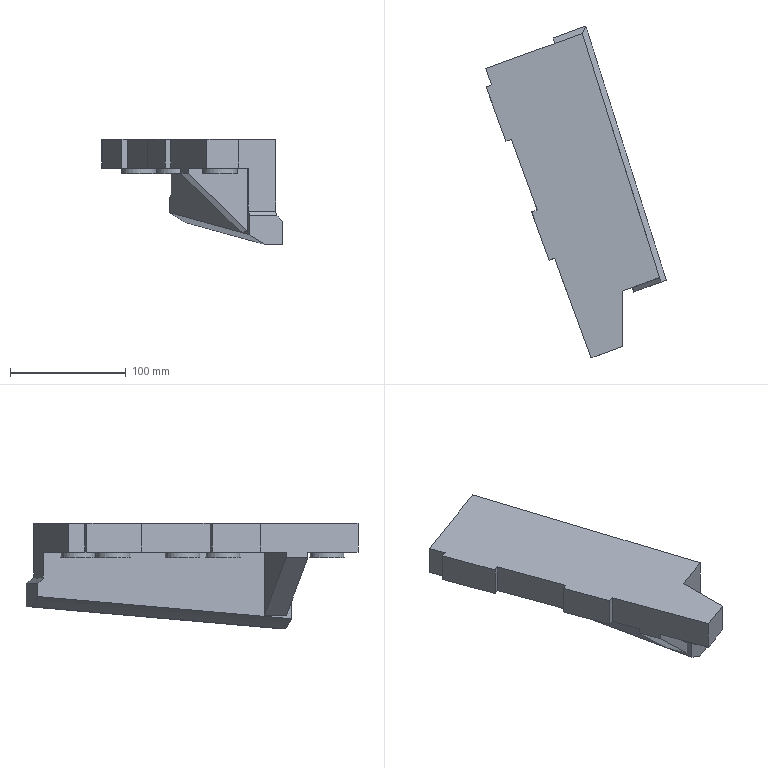Part | NX | features solid 2 | 1 solid | 40 faces | box 156.114 x 286.817 x 91.178 mm | volume 898598 mm3 | plane 29 | spline 6 | cylinder 5 | commonest cylinder face diameters 30 x5